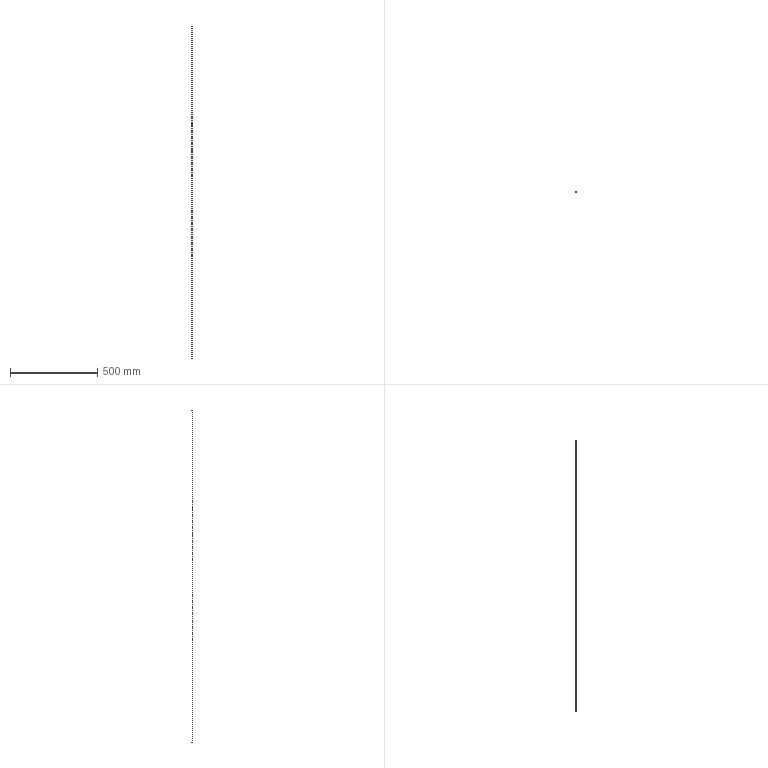Part | SolidWorks | features Extrusion 1 | 1 solid | 4 faces | box 0.125 x 0.125 x 1900 mm | volume 23.317 mm3 | cylinder 2 | plane 2 | commonest cylinder face diameters 0.125 x2
STEP:
#1=CARTESIAN_POINT('',(0.0625,0.,1900.));
#2=VERTEX_POINT('',#1);
#3=CARTESIAN_POINT('',(-0.0625,0.,1900.));
#4=VERTEX_POINT('',#3);
#5=CARTESIAN_POINT('',(0.,0.,1900.));
#6=DIRECTION('',(0.,0.,1.));
#7=DIRECTION('',(1.,0.,0.));
#8=AXIS2_PLACEMENT_3D('',#5,#6,#7);
#9=CIRCLE('',#8,0.0625);
#10=EDGE_CURVE('',#2,#4,#9,.T.);
#11=ORIENTED_EDGE('',*,*,#10,.F.);
#12=CARTESIAN_POINT('',(0.0625,0.,0.));
#13=VERTEX_POINT('',#12);
#14=CARTESIAN_POINT('',(0.0625,0.,1900.));
#15=DIRECTION('',(0.,0.,-1.));
#16=VECTOR('',#15,1000.);
#17=LINE('',#14,#16);
#18=EDGE_CURVE('',#2,#13,#17,.T.);
#19=ORIENTED_EDGE('',*,*,#18,.T.);
#20=CARTESIAN_POINT('',(-0.0625,0.,0.));
#21=VERTEX_POINT('',#20);
#22=CARTESIAN_POINT('',(0.,0.,0.));
#23=DIRECTION('',(0.,0.,1.));
#24=DIRECTION('',(1.,0.,0.));
#25=AXIS2_PLACEMENT_3D('',#22,#23,#24);
#26=CIRCLE('',#25,0.0625);
#27=EDGE_CURVE('',#13,#21,#26,.T.);
#28=ORIENTED_EDGE('',*,*,#27,.T.);
#29=CARTESIAN_POINT('',(-0.0625,0.,1900.));
#30=DIRECTION('',(0.,0.,-1.));
#31=VECTOR('',#30,1000.);
#32=LINE('',#29,#31);
#33=EDGE_CURVE('',#4,#21,#32,.T.);
#34=ORIENTED_EDGE('',*,*,#33,.F.);
#35=EDGE_LOOP('',(#11,#19,#28,#34));
#36=FACE_OUTER_BOUND('',#35,.T.);
#37=CARTESIAN_POINT('',(0.,0.,1900.));
#38=DIRECTION('',(0.,0.,-1.));
#39=DIRECTION('',(-1.,0.,0.));
#40=AXIS2_PLACEMENT_3D('',#37,#38,#39);
#41=CYLINDRICAL_SURFACE('',#40,0.0625);
#42=ADVANCED_FACE('',(#36),#41,.T.);
#43=ORIENTED_EDGE('',*,*,#18,.F.);
#44=CARTESIAN_POINT('',(0.,0.,1900.));
#45=DIRECTION('',(0.,0.,1.));
#46=DIRECTION('',(1.,0.,0.));
#47=AXIS2_PLACEMENT_3D('',#44,#45,#46);
#48=CIRCLE('',#47,0.0625);
#49=EDGE_CURVE('',#4,#2,#48,.T.);
#50=ORIENTED_EDGE('',*,*,#49,.F.);
#51=ORIENTED_EDGE('',*,*,#33,.T.);
#52=CARTESIAN_POINT('',(0.,0.,0.));
#53=DIRECTION('',(0.,0.,1.));
#54=DIRECTION('',(1.,0.,0.));
#55=AXIS2_PLACEMENT_3D('',#52,#53,#54);
#56=CIRCLE('',#55,0.0625);
#57=EDGE_CURVE('',#21,#13,#56,.T.);
#58=ORIENTED_EDGE('',*,*,#57,.T.);
#59=EDGE_LOOP('',(#43,#50,#51,#58));
#60=FACE_OUTER_BOUND('',#59,.T.);
#61=CARTESIAN_POINT('',(0.,0.,1900.));
#62=DIRECTION('',(0.,0.,-1.));
#63=DIRECTION('',(-1.,0.,0.));
#64=AXIS2_PLACEMENT_3D('',#61,#62,#63);
#65=CYLINDRICAL_SURFACE('',#64,0.0625);
#66=ADVANCED_FACE('',(#60),#65,.T.);
#67=ORIENTED_EDGE('',*,*,#49,.T.);
#68=ORIENTED_EDGE('',*,*,#10,.T.);
#69=EDGE_LOOP('',(#67,#68));
#70=FACE_OUTER_BOUND('',#69,.T.);
#71=CARTESIAN_POINT('',(0.,0.,1900.));
#72=DIRECTION('',(0.,0.,1.));
#73=DIRECTION('',(1.,0.,0.));
#74=AXIS2_PLACEMENT_3D('',#71,#72,#73);
#75=PLANE('',#74);
#76=ADVANCED_FACE('',(#70),#75,.T.);
#77=ORIENTED_EDGE('',*,*,#57,.F.);
#78=ORIENTED_EDGE('',*,*,#27,.F.);
#79=EDGE_LOOP('',(#77,#78));
#80=FACE_OUTER_BOUND('',#79,.T.);
#81=CARTESIAN_POINT('',(0.,0.,0.));
#82=DIRECTION('',(0.,0.,1.));
#83=DIRECTION('',(1.,0.,0.));
#84=AXIS2_PLACEMENT_3D('',#81,#82,#83);
#85=PLANE('',#84);
#86=ADVANCED_FACE('',(#80),#85,.F.);
#87=CLOSED_SHELL('',(#42,#66,#76,#86));
#88=MANIFOLD_SOLID_BREP('',#87);
#89=CARTESIAN_POINT('',(0.,0.,0.));
#90=DIRECTION('',(0.,0.,1.));
#91=DIRECTION('',(1.,0.,0.));
#92=AXIS2_PLACEMENT_3D('',#89,#90,#91);
#93=(LENGTH_UNIT()NAMED_UNIT(*)SI_UNIT(.MILLI.,.METRE.));
#94=UNCERTAINTY_MEASURE_WITH_UNIT(LENGTH_MEASURE(0.00001),#93,'','');
#95=(NAMED_UNIT(*)PLANE_ANGLE_UNIT()SI_UNIT($,.RADIAN.));
#96=(NAMED_UNIT(*)SI_UNIT($,.STERADIAN.)SOLID_ANGLE_UNIT());
#97=(GEOMETRIC_REPRESENTATION_CONTEXT(3)GLOBAL_UNCERTAINTY_ASSIGNED_CONTEXT((#94))GLOBAL_UNIT_ASSIGNED_CONTEXT((#93,#95,#96))REPRESENTATION_CONTEXT('',''));
#98=ADVANCED_BREP_SHAPE_REPRESENTATION('',(#88,#92),#97);